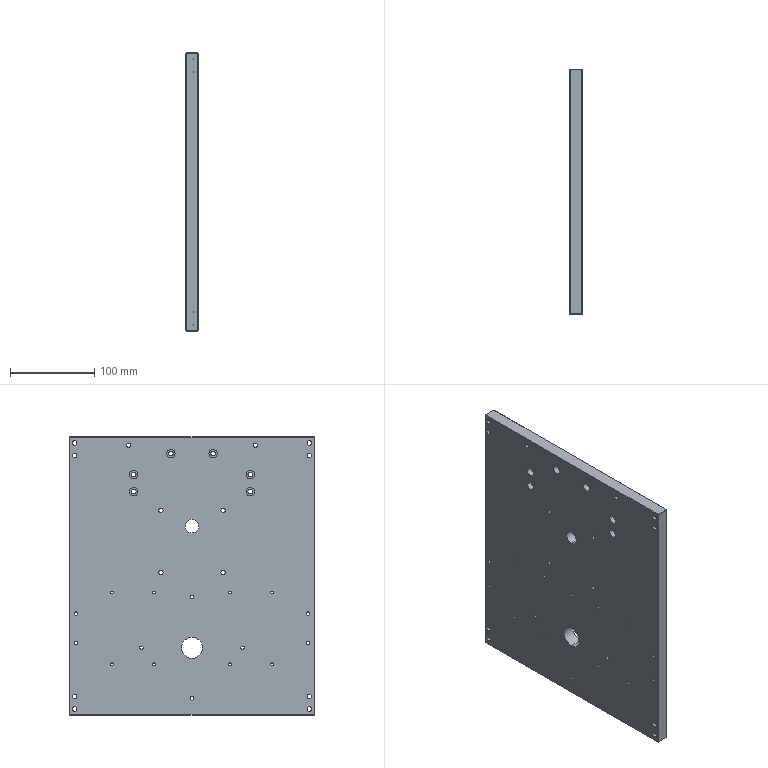Part | STEP file | 06-18 Fixing plate 1 | 1 solid | 144 faces | box 15 x 290 x 330 mm | volume 1410593 mm3 | cylinder 104 | plane 40 | commonest cylinder face diameters 5.5 x28 10 x28 3.3 x16 4.2 x16 5 x12 16 x2